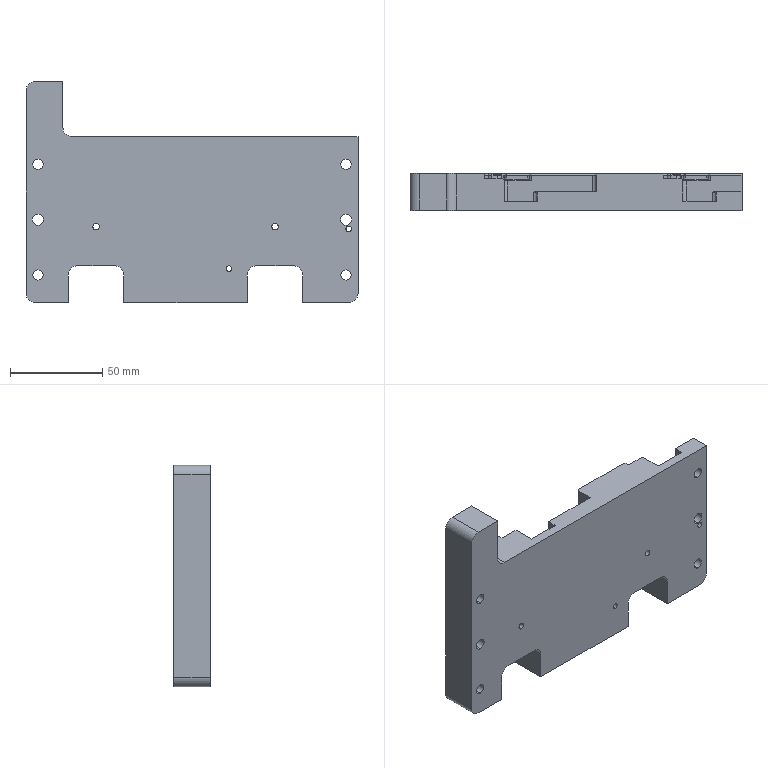Part | STEP file | 04-01 left bending base die | 1 solid | 456 faces | box 180 x 20 x 120 mm | volume 264352 mm3 | plane 190 | cylinder 183 | cone 55 | torus 20 | sphere 8 | commonest cylinder face diameters 2 x70 3 x22 4 x19 10 x16 2.5 x12 3.1 x12